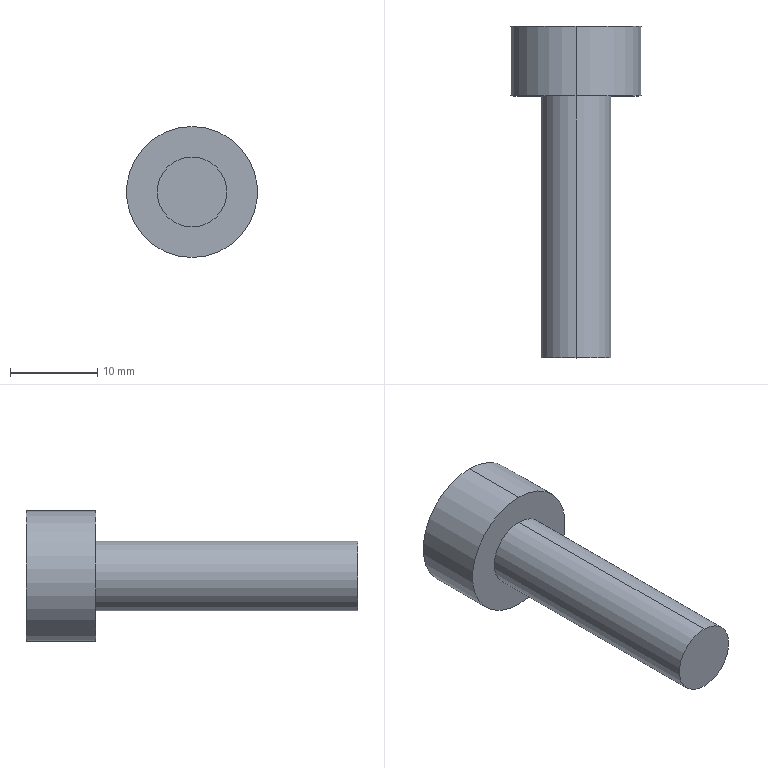Part | STEP file | 1 solid | 14 faces | box 15 x 38 x 15 mm | volume 2735 mm3 | plane 10 | cylinder 4 | commonest cylinder face diameters 8 x2 15 x2
STEP:
#1=CARTESIAN_POINT('',(0.,0.,0.));
#2=DIRECTION('',(0.,0.,1.));
#3=DIRECTION('',(1.,0.,0.));
#4=AXIS2_PLACEMENT_3D('',#1,#2,#3);
#5=CARTESIAN_POINT('',(0.,38.,-7.5));
#6=VERTEX_POINT('',#5);
#7=CARTESIAN_POINT('',(0.,38.,7.5));
#8=VERTEX_POINT('',#7);
#9=CARTESIAN_POINT('',(0.,38.,0.));
#10=DIRECTION('',(0.,-1.,0.));
#11=DIRECTION('',(0.,0.,-1.));
#12=AXIS2_PLACEMENT_3D('',#9,#10,#11);
#13=CIRCLE('',#12,7.5);
#14=CARTESIAN_POINT('',(0.,0.,0.));
#15=DIRECTION('',(0.,-1.,0.));
#16=DIRECTION('',(0.,0.,-1.));
#17=AXIS2_PLACEMENT_3D('',#14,#15,#16);
#18=CYLINDRICAL_SURFACE('',#17,7.5);
#19=CARTESIAN_POINT('',(0.,-38.));
#20=DIRECTION('',(1.,0.));
#21=VECTOR('',#20,1.);
#22=LINE('',#19,#21);
#23=(GEOMETRIC_REPRESENTATION_CONTEXT(2)PARAMETRIC_REPRESENTATION_CONTEXT()REPRESENTATION_CONTEXT('',''));
#24=DEFINITIONAL_REPRESENTATION('',(#22),#23);
#25=PCURVE('',#18,#24);
#26=CARTESIAN_POINT('',(7.5,38.,0.));
#27=DIRECTION('',(0.,1.,0.));
#28=DIRECTION('',(0.,0.,1.));
#29=AXIS2_PLACEMENT_3D('',#26,#27,#28);
#30=PLANE('',#29);
#31=CARTESIAN_POINT('',(-7.5,-7.5));
#32=CARTESIAN_POINT('',(-7.5,5.49));
#33=CARTESIAN_POINT('',(3.75,-1.005));
#34=CARTESIAN_POINT('',(15.,-7.5));
#35=CARTESIAN_POINT('',(3.75,-13.995));
#36=CARTESIAN_POINT('',(-7.5,-20.49));
#37=CARTESIAN_POINT('',(-7.5,-7.5));
#38=(BOUNDED_CURVE()B_SPLINE_CURVE(2,(#31,#32,#33,#34,#35,#36,#37),.UNSPECIFIED.,.T.,.F.)B_SPLINE_CURVE_WITH_KNOTS((1,2,2,2,2,1),(-2.094,0.,2.094,4.189,6.283,8.378),.UNSPECIFIED.)CURVE()GEOMETRIC_REPRESENTATION_ITEM()RATIONAL_B_SPLINE_CURVE((1.,0.5,1.,0.5,1.,0.5,1.))REPRESENTATION_ITEM(''));
#39=(GEOMETRIC_REPRESENTATION_CONTEXT(2)PARAMETRIC_REPRESENTATION_CONTEXT()REPRESENTATION_CONTEXT('',''));
#40=DEFINITIONAL_REPRESENTATION('',(#38),#39);
#41=PCURVE('',#30,#40);
#42=SURFACE_CURVE('',#13,(#25,#41),.PCURVE_S1.);
#43=EDGE_CURVE('',#6,#8,#42,.T.);
#44=ORIENTED_EDGE('',*,*,#43,.T.);
#45=CARTESIAN_POINT('',(0.,30.,7.5));
#46=VERTEX_POINT('',#45);
#47=CARTESIAN_POINT('',(0.,0.,7.5));
#48=DIRECTION('',(0.,-1.,0.));
#49=VECTOR('',#48,1.);
#50=LINE('',#47,#49);
#51=CARTESIAN_POINT('',(3.142,0.));
#52=DIRECTION('',(0.,1.));
#53=VECTOR('',#52,1.);
#54=LINE('',#51,#53);
#55=(GEOMETRIC_REPRESENTATION_CONTEXT(2)PARAMETRIC_REPRESENTATION_CONTEXT()REPRESENTATION_CONTEXT('',''));
#56=DEFINITIONAL_REPRESENTATION('',(#54),#55);
#57=PCURVE('',#18,#56);
#58=CARTESIAN_POINT('',(0.,0.,0.));
#59=DIRECTION('',(0.,-1.,0.));
#60=DIRECTION('',(0.,0.,-1.));
#61=AXIS2_PLACEMENT_3D('',#58,#59,#60);
#62=CYLINDRICAL_SURFACE('',#61,7.5);
#63=CARTESIAN_POINT('',(3.142,0.));
#64=DIRECTION('',(0.,1.));
#65=VECTOR('',#64,1.);
#66=LINE('',#63,#65);
#67=(GEOMETRIC_REPRESENTATION_CONTEXT(2)PARAMETRIC_REPRESENTATION_CONTEXT()REPRESENTATION_CONTEXT('',''));
#68=DEFINITIONAL_REPRESENTATION('',(#66),#67);
#69=PCURVE('',#62,#68);
#70=SURFACE_CURVE('',#50,(#57,#69),.PCURVE_S1.);
#71=EDGE_CURVE('',#8,#46,#70,.T.);
#72=ORIENTED_EDGE('',*,*,#71,.T.);
#73=CARTESIAN_POINT('',(0.,30.,-7.5));
#74=VERTEX_POINT('',#73);
#75=CARTESIAN_POINT('',(0.,30.,0.));
#76=DIRECTION('',(0.,-1.,0.));
#77=DIRECTION('',(0.,0.,-1.));
#78=AXIS2_PLACEMENT_3D('',#75,#76,#77);
#79=CIRCLE('',#78,7.5);
#80=CARTESIAN_POINT('',(0.,-30.));
#81=DIRECTION('',(1.,0.));
#82=VECTOR('',#81,1.);
#83=LINE('',#80,#82);
#84=(GEOMETRIC_REPRESENTATION_CONTEXT(2)PARAMETRIC_REPRESENTATION_CONTEXT()REPRESENTATION_CONTEXT('',''));
#85=DEFINITIONAL_REPRESENTATION('',(#83),#84);
#86=PCURVE('',#18,#85);
#87=CARTESIAN_POINT('',(4.,30.,0.));
#88=DIRECTION('',(0.,-1.,0.));
#89=DIRECTION('',(0.,0.,-1.));
#90=AXIS2_PLACEMENT_3D('',#87,#88,#89);
#91=PLANE('',#90);
#92=CARTESIAN_POINT('',(0.,-4.));
#93=DIRECTION('',(1.,0.));
#94=AXIS2_PLACEMENT_2D('',#92,#93);
#95=CIRCLE('',#94,7.5);
#96=(GEOMETRIC_REPRESENTATION_CONTEXT(2)PARAMETRIC_REPRESENTATION_CONTEXT()REPRESENTATION_CONTEXT('',''));
#97=DEFINITIONAL_REPRESENTATION('',(#95),#96);
#98=PCURVE('',#91,#97);
#99=SURFACE_CURVE('',#79,(#86,#98),.PCURVE_S1.);
#100=EDGE_CURVE('',#74,#46,#99,.T.);
#101=ORIENTED_EDGE('',*,*,#100,.F.);
#102=CARTESIAN_POINT('',(0.,0.,-7.5));
#103=DIRECTION('',(0.,-1.,0.));
#104=VECTOR('',#103,1.);
#105=LINE('',#102,#104);
#106=CARTESIAN_POINT('',(0.,0.));
#107=DIRECTION('',(0.,1.));
#108=VECTOR('',#107,1.);
#109=LINE('',#106,#108);
#110=(GEOMETRIC_REPRESENTATION_CONTEXT(2)PARAMETRIC_REPRESENTATION_CONTEXT()REPRESENTATION_CONTEXT('',''));
#111=DEFINITIONAL_REPRESENTATION('',(#109),#110);
#112=PCURVE('',#18,#111);
#113=CARTESIAN_POINT('',(6.283,0.));
#114=DIRECTION('',(0.,1.));
#115=VECTOR('',#114,1.);
#116=LINE('',#113,#115);
#117=(GEOMETRIC_REPRESENTATION_CONTEXT(2)PARAMETRIC_REPRESENTATION_CONTEXT()REPRESENTATION_CONTEXT('',''));
#118=DEFINITIONAL_REPRESENTATION('',(#116),#117);
#119=PCURVE('',#62,#118);
#120=SURFACE_CURVE('',#105,(#112,#119),.PCURVE_S1.);
#121=EDGE_CURVE('',#6,#74,#120,.T.);
#122=ORIENTED_EDGE('',*,*,#121,.F.);
#123=EDGE_LOOP('',(#44,#72,#101,#122));
#124=FACE_BOUND('',#123,.T.);
#125=ADVANCED_FACE('',(#124),#18,.T.);
#126=CARTESIAN_POINT('',(0.,30.,-4.));
#127=VERTEX_POINT('',#126);
#128=CARTESIAN_POINT('',(0.,30.,4.));
#129=VERTEX_POINT('',#128);
#130=CARTESIAN_POINT('',(0.,30.,0.));
#131=DIRECTION('',(0.,-1.,0.));
#132=DIRECTION('',(0.,0.,-1.));
#133=AXIS2_PLACEMENT_3D('',#130,#131,#132);
#134=CIRCLE('',#133,4.);
#135=CARTESIAN_POINT('',(0.,0.,0.));
#136=DIRECTION('',(0.,-1.,0.));
#137=DIRECTION('',(0.,0.,-1.));
#138=AXIS2_PLACEMENT_3D('',#135,#136,#137);
#139=CYLINDRICAL_SURFACE('',#138,4.);
#140=CARTESIAN_POINT('',(0.,-30.));
#141=DIRECTION('',(1.,0.));
#142=VECTOR('',#141,1.);
#143=LINE('',#140,#142);
#144=(GEOMETRIC_REPRESENTATION_CONTEXT(2)PARAMETRIC_REPRESENTATION_CONTEXT()REPRESENTATION_CONTEXT('',''));
#145=DEFINITIONAL_REPRESENTATION('',(#143),#144);
#146=PCURVE('',#139,#145);
#147=CARTESIAN_POINT('',(0.,-4.));
#148=DIRECTION('',(1.,0.));
#149=AXIS2_PLACEMENT_2D('',#147,#148);
#150=CIRCLE('',#149,4.);
#151=(GEOMETRIC_REPRESENTATION_CONTEXT(2)PARAMETRIC_REPRESENTATION_CONTEXT()REPRESENTATION_CONTEXT('',''));
#152=DEFINITIONAL_REPRESENTATION('',(#150),#151);
#153=PCURVE('',#91,#152);
#154=SURFACE_CURVE('',#134,(#146,#153),.PCURVE_S1.);
#155=EDGE_CURVE('',#127,#129,#154,.T.);
#156=ORIENTED_EDGE('',*,*,#155,.T.);
#157=CARTESIAN_POINT('',(0.,0.,4.));
#158=VERTEX_POINT('',#157);
#159=CARTESIAN_POINT('',(0.,0.,4.));
#160=DIRECTION('',(0.,-1.,0.));
#161=VECTOR('',#160,1.);
#162=LINE('',#159,#161);
#163=CARTESIAN_POINT('',(3.142,0.));
#164=DIRECTION('',(0.,1.));
#165=VECTOR('',#164,1.);
#166=LINE('',#163,#165);
#167=(GEOMETRIC_REPRESENTATION_CONTEXT(2)PARAMETRIC_REPRESENTATION_CONTEXT()REPRESENTATION_CONTEXT('',''));
#168=DEFINITIONAL_REPRESENTATION('',(#166),#167);
#169=PCURVE('',#139,#168);
#170=CARTESIAN_POINT('',(0.,0.,0.));
#171=DIRECTION('',(0.,-1.,0.));
#172=DIRECTION('',(0.,0.,-1.));
#173=AXIS2_PLACEMENT_3D('',#170,#171,#172);
#174=CYLINDRICAL_SURFACE('',#173,4.);
#175=CARTESIAN_POINT('',(3.142,0.));
#176=DIRECTION('',(0.,1.));
#177=VECTOR('',#176,1.);
#178=LINE('',#175,#177);
#179=(GEOMETRIC_REPRESENTATION_CONTEXT(2)PARAMETRIC_REPRESENTATION_CONTEXT()REPRESENTATION_CONTEXT('',''));
#180=DEFINITIONAL_REPRESENTATION('',(#178),#179);
#181=PCURVE('',#174,#180);
#182=SURFACE_CURVE('',#162,(#169,#181),.PCURVE_S1.);
#183=EDGE_CURVE('',#129,#158,#182,.T.);
#184=ORIENTED_EDGE('',*,*,#183,.T.);
#185=CARTESIAN_POINT('',(0.,0.,-4.));
#186=VERTEX_POINT('',#185);
#187=CARTESIAN_POINT('',(0.,0.,0.));
#188=DIRECTION('',(0.,-1.,0.));
#189=DIRECTION('',(0.,0.,-1.));
#190=AXIS2_PLACEMENT_3D('',#187,#188,#189);
#191=CIRCLE('',#190,4.);
#192=CARTESIAN_POINT('',(0.,0.));
#193=DIRECTION('',(1.,0.));
#194=VECTOR('',#193,1.);
#195=LINE('',#192,#194);
#196=(GEOMETRIC_REPRESENTATION_CONTEXT(2)PARAMETRIC_REPRESENTATION_CONTEXT()REPRESENTATION_CONTEXT('',''));
#197=DEFINITIONAL_REPRESENTATION('',(#195),#196);
#198=PCURVE('',#139,#197);
#199=CARTESIAN_POINT('',(0.,0.,0.));
#200=DIRECTION('',(0.,-1.,0.));
#201=DIRECTION('',(0.,0.,-1.));
#202=AXIS2_PLACEMENT_3D('',#199,#200,#201);
#203=PLANE('',#202);
#204=CARTESIAN_POINT('',(0.,0.));
#205=DIRECTION('',(1.,0.));
#206=AXIS2_PLACEMENT_2D('',#204,#205);
#207=CIRCLE('',#206,4.);
#208=(GEOMETRIC_REPRESENTATION_CONTEXT(2)PARAMETRIC_REPRESENTATION_CONTEXT()REPRESENTATION_CONTEXT('',''));
#209=DEFINITIONAL_REPRESENTATION('',(#207),#208);
#210=PCURVE('',#203,#209);
#211=SURFACE_CURVE('',#191,(#198,#210),.PCURVE_S1.);
#212=EDGE_CURVE('',#186,#158,#211,.T.);
#213=ORIENTED_EDGE('',*,*,#212,.F.);
#214=CARTESIAN_POINT('',(0.,0.,-4.));
#215=DIRECTION('',(0.,-1.,0.));
#216=VECTOR('',#215,1.);
#217=LINE('',#214,#216);
#218=CARTESIAN_POINT('',(0.,0.));
#219=DIRECTION('',(0.,1.));
#220=VECTOR('',#219,1.);
#221=LINE('',#218,#220);
#222=(GEOMETRIC_REPRESENTATION_CONTEXT(2)PARAMETRIC_REPRESENTATION_CONTEXT()REPRESENTATION_CONTEXT('',''));
#223=DEFINITIONAL_REPRESENTATION('',(#221),#222);
#224=PCURVE('',#139,#223);
#225=CARTESIAN_POINT('',(6.283,0.));
#226=DIRECTION('',(0.,1.));
#227=VECTOR('',#226,1.);
#228=LINE('',#225,#227);
#229=(GEOMETRIC_REPRESENTATION_CONTEXT(2)PARAMETRIC_REPRESENTATION_CONTEXT()REPRESENTATION_CONTEXT('',''));
#230=DEFINITIONAL_REPRESENTATION('',(#228),#229);
#231=PCURVE('',#174,#230);
#232=SURFACE_CURVE('',#217,(#224,#231),.PCURVE_S1.);
#233=EDGE_CURVE('',#127,#186,#232,.T.);
#234=ORIENTED_EDGE('',*,*,#233,.F.);
#235=EDGE_LOOP('',(#156,#184,#213,#234));
#236=FACE_BOUND('',#235,.T.);
#237=ADVANCED_FACE('',(#236),#139,.T.);
#238=ORIENTED_EDGE('',*,*,#212,.T.);
#239=CARTESIAN_POINT('',(0.,0.,0.));
#240=DIRECTION('',(0.,-1.,0.));
#241=DIRECTION('',(0.,0.,-1.));
#242=AXIS2_PLACEMENT_3D('',#239,#240,#241);
#243=CIRCLE('',#242,4.);
#244=CARTESIAN_POINT('',(0.,0.));
#245=DIRECTION('',(1.,0.));
#246=AXIS2_PLACEMENT_2D('',#244,#245);
#247=CIRCLE('',#246,4.);
#248=(GEOMETRIC_REPRESENTATION_CONTEXT(2)PARAMETRIC_REPRESENTATION_CONTEXT()REPRESENTATION_CONTEXT('',''));
#249=DEFINITIONAL_REPRESENTATION('',(#247),#248);
#250=PCURVE('',#203,#249);
#251=CARTESIAN_POINT('',(0.,0.));
#252=DIRECTION('',(1.,0.));
#253=VECTOR('',#252,1.);
#254=LINE('',#251,#253);
#255=(GEOMETRIC_REPRESENTATION_CONTEXT(2)PARAMETRIC_REPRESENTATION_CONTEXT()REPRESENTATION_CONTEXT('',''));
#256=DEFINITIONAL_REPRESENTATION('',(#254),#255);
#257=PCURVE('',#174,#256);
#258=SURFACE_CURVE('',#243,(#250,#257),.PCURVE_S1.);
#259=EDGE_CURVE('',#158,#186,#258,.T.);
#260=ORIENTED_EDGE('',*,*,#259,.T.);
#261=EDGE_LOOP('',(#238,#260));
#262=FACE_BOUND('',#261,.T.);
#263=ADVANCED_FACE('',(#262),#203,.T.);
#264=ORIENTED_EDGE('',*,*,#183,.F.);
#265=CARTESIAN_POINT('',(0.,30.,0.));
#266=DIRECTION('',(0.,-1.,0.));
#267=DIRECTION('',(0.,0.,-1.));
#268=AXIS2_PLACEMENT_3D('',#265,#266,#267);
#269=CIRCLE('',#268,4.);
#270=CARTESIAN_POINT('',(0.,-30.));
#271=DIRECTION('',(1.,0.));
#272=VECTOR('',#271,1.);
#273=LINE('',#270,#272);
#274=(GEOMETRIC_REPRESENTATION_CONTEXT(2)PARAMETRIC_REPRESENTATION_CONTEXT()REPRESENTATION_CONTEXT('',''));
#275=DEFINITIONAL_REPRESENTATION('',(#273),#274);
#276=PCURVE('',#174,#275);
#277=CARTESIAN_POINT('',(0.,-4.));
#278=DIRECTION('',(1.,0.));
#279=AXIS2_PLACEMENT_2D('',#277,#278);
#280=CIRCLE('',#279,4.);
#281=(GEOMETRIC_REPRESENTATION_CONTEXT(2)PARAMETRIC_REPRESENTATION_CONTEXT()REPRESENTATION_CONTEXT('',''));
#282=DEFINITIONAL_REPRESENTATION('',(#280),#281);
#283=PCURVE('',#91,#282);
#284=SURFACE_CURVE('',#269,(#276,#283),.PCURVE_S1.);
#285=EDGE_CURVE('',#129,#127,#284,.T.);
#286=ORIENTED_EDGE('',*,*,#285,.T.);
#287=ORIENTED_EDGE('',*,*,#233,.T.);
#288=ORIENTED_EDGE('',*,*,#259,.F.);
#289=EDGE_LOOP('',(#264,#286,#287,#288));
#290=FACE_BOUND('',#289,.T.);
#291=ADVANCED_FACE('',(#290),#174,.T.);
#292=ORIENTED_EDGE('',*,*,#100,.T.);
#293=CARTESIAN_POINT('',(0.,30.,0.));
#294=DIRECTION('',(0.,-1.,0.));
#295=DIRECTION('',(0.,0.,-1.));
#296=AXIS2_PLACEMENT_3D('',#293,#294,#295);
#297=CIRCLE('',#296,7.5);
#298=CARTESIAN_POINT('',(0.,-4.));
#299=DIRECTION('',(1.,0.));
#300=AXIS2_PLACEMENT_2D('',#298,#299);
#301=CIRCLE('',#300,7.5);
#302=(GEOMETRIC_REPRESENTATION_CONTEXT(2)PARAMETRIC_REPRESENTATION_CONTEXT()REPRESENTATION_CONTEXT('',''));
#303=DEFINITIONAL_REPRESENTATION('',(#301),#302);
#304=PCURVE('',#91,#303);
#305=CARTESIAN_POINT('',(0.,-30.));
#306=DIRECTION('',(1.,0.));
#307=VECTOR('',#306,1.);
#308=LINE('',#305,#307);
#309=(GEOMETRIC_REPRESENTATION_CONTEXT(2)PARAMETRIC_REPRESENTATION_CONTEXT()REPRESENTATION_CONTEXT('',''));
#310=DEFINITIONAL_REPRESENTATION('',(#308),#309);
#311=PCURVE('',#62,#310);
#312=SURFACE_CURVE('',#297,(#304,#311),.PCURVE_S1.);
#313=EDGE_CURVE('',#46,#74,#312,.T.);
#314=ORIENTED_EDGE('',*,*,#313,.T.);
#315=EDGE_LOOP('',(#292,#314));
#316=FACE_BOUND('',#315,.T.);
#317=ORIENTED_EDGE('',*,*,#155,.F.);
#318=ORIENTED_EDGE('',*,*,#285,.F.);
#319=EDGE_LOOP('',(#317,#318));
#320=FACE_BOUND('',#319,.T.);
#321=ADVANCED_FACE('',(#316,#320),#91,.T.);
#322=ORIENTED_EDGE('',*,*,#71,.F.);
#323=CARTESIAN_POINT('',(0.,38.,0.));
#324=DIRECTION('',(0.,-1.,0.));
#325=DIRECTION('',(0.,0.,-1.));
#326=AXIS2_PLACEMENT_3D('',#323,#324,#325);
#327=CIRCLE('',#326,7.5);
#328=CARTESIAN_POINT('',(0.,-38.));
#329=DIRECTION('',(1.,0.));
#330=VECTOR('',#329,1.);
#331=LINE('',#328,#330);
#332=(GEOMETRIC_REPRESENTATION_CONTEXT(2)PARAMETRIC_REPRESENTATION_CONTEXT()REPRESENTATION_CONTEXT('',''));
#333=DEFINITIONAL_REPRESENTATION('',(#331),#332);
#334=PCURVE('',#62,#333);
#335=CARTESIAN_POINT('',(-7.5,-7.5));
#336=CARTESIAN_POINT('',(-7.5,5.49));
#337=CARTESIAN_POINT('',(3.75,-1.005));
#338=CARTESIAN_POINT('',(15.,-7.5));
#339=CARTESIAN_POINT('',(3.75,-13.995));
#340=CARTESIAN_POINT('',(-7.5,-20.49));
#341=CARTESIAN_POINT('',(-7.5,-7.5));
#342=(BOUNDED_CURVE()B_SPLINE_CURVE(2,(#335,#336,#337,#338,#339,#340,#341),.UNSPECIFIED.,.T.,.F.)B_SPLINE_CURVE_WITH_KNOTS((1,2,2,2,2,1),(-2.094,0.,2.094,4.189,6.283,8.378),.UNSPECIFIED.)CURVE()GEOMETRIC_REPRESENTATION_ITEM()RATIONAL_B_SPLINE_CURVE((1.,0.5,1.,0.5,1.,0.5,1.))REPRESENTATION_ITEM(''));
#343=(GEOMETRIC_REPRESENTATION_CONTEXT(2)PARAMETRIC_REPRESENTATION_CONTEXT()REPRESENTATION_CONTEXT('',''));
#344=DEFINITIONAL_REPRESENTATION('',(#342),#343);
#345=PCURVE('',#30,#344);
#346=SURFACE_CURVE('',#327,(#334,#345),.PCURVE_S1.);
#347=EDGE_CURVE('',#8,#6,#346,.T.);
#348=ORIENTED_EDGE('',*,*,#347,.T.);
#349=ORIENTED_EDGE('',*,*,#121,.T.);
#350=ORIENTED_EDGE('',*,*,#313,.F.);
#351=EDGE_LOOP('',(#322,#348,#349,#350));
#352=FACE_BOUND('',#351,.T.);
#353=ADVANCED_FACE('',(#352),#62,.T.);
#354=CARTESIAN_POINT('',(1.732,38.,3.));
#355=VERTEX_POINT('',#354);
#356=CARTESIAN_POINT('',(3.464,38.,0.));
#357=VERTEX_POINT('',#356);
#358=CARTESIAN_POINT('',(1.732,38.,3.));
#359=DIRECTION('',(0.5,0.,-0.866));
#360=VECTOR('',#359,1.);
#361=LINE('',#358,#360);
#362=CARTESIAN_POINT('',(3.,-5.768));
#363=DIRECTION('',(-0.866,0.5));
#364=VECTOR('',#363,1.);
#365=LINE('',#362,#364);
#366=(GEOMETRIC_REPRESENTATION_CONTEXT(2)PARAMETRIC_REPRESENTATION_CONTEXT()REPRESENTATION_CONTEXT('',''));
#367=DEFINITIONAL_REPRESENTATION('',(#365),#366);
#368=PCURVE('',#30,#367);
#369=CARTESIAN_POINT('',(1.732,32.,3.));
#370=DIRECTION('',(0.866,0.,0.5));
#371=DIRECTION('',(0.5,0.,-0.866));
#372=AXIS2_PLACEMENT_3D('',#369,#370,#371);
#373=PLANE('',#372);
#374=CARTESIAN_POINT('',(0.,6.));
#375=DIRECTION('',(1.,0.));
#376=VECTOR('',#375,1.);
#377=LINE('',#374,#376);
#378=(GEOMETRIC_REPRESENTATION_CONTEXT(2)PARAMETRIC_REPRESENTATION_CONTEXT()REPRESENTATION_CONTEXT('',''));
#379=DEFINITIONAL_REPRESENTATION('',(#377),#378);
#380=PCURVE('',#373,#379);
#381=SURFACE_CURVE('',#361,(#368,#380),.PCURVE_S1.);
#382=EDGE_CURVE('',#355,#357,#381,.T.);
#383=ORIENTED_EDGE('',*,*,#382,.F.);
#384=CARTESIAN_POINT('',(-1.732,38.,3.));
#385=VERTEX_POINT('',#384);
#386=CARTESIAN_POINT('',(-1.732,38.,3.));
#387=DIRECTION('',(1.,0.,0.));
#388=VECTOR('',#387,1.);
#389=LINE('',#386,#388);
#390=CARTESIAN_POINT('',(3.,-9.232));
#391=DIRECTION('',(0.,1.));
#392=VECTOR('',#391,1.);
#393=LINE('',#390,#392);
#394=(GEOMETRIC_REPRESENTATION_CONTEXT(2)PARAMETRIC_REPRESENTATION_CONTEXT()REPRESENTATION_CONTEXT('',''));
#395=DEFINITIONAL_REPRESENTATION('',(#393),#394);
#396=PCURVE('',#30,#395);
#397=CARTESIAN_POINT('',(-1.732,32.,3.));
#398=DIRECTION('',(0.,0.,1.));
#399=DIRECTION('',(1.,0.,0.));
#400=AXIS2_PLACEMENT_3D('',#397,#398,#399);
#401=PLANE('',#400);
#402=CARTESIAN_POINT('',(0.,6.));
#403=DIRECTION('',(1.,0.));
#404=VECTOR('',#403,1.);
#405=LINE('',#402,#404);
#406=(GEOMETRIC_REPRESENTATION_CONTEXT(2)PARAMETRIC_REPRESENTATION_CONTEXT()REPRESENTATION_CONTEXT('',''));
#407=DEFINITIONAL_REPRESENTATION('',(#405),#406);
#408=PCURVE('',#401,#407);
#409=SURFACE_CURVE('',#389,(#396,#408),.PCURVE_S1.);
#410=EDGE_CURVE('',#385,#355,#409,.T.);
#411=ORIENTED_EDGE('',*,*,#410,.F.);
#412=CARTESIAN_POINT('',(-3.464,38.,0.));
#413=VERTEX_POINT('',#412);
#414=CARTESIAN_POINT('',(-3.464,38.,0.));
#415=DIRECTION('',(0.5,0.,0.866));
#416=VECTOR('',#415,1.);
#417=LINE('',#414,#416);
#418=CARTESIAN_POINT('',(0.,-10.964));
#419=DIRECTION('',(0.866,0.5));
#420=VECTOR('',#419,1.);
#421=LINE('',#418,#420);
#422=(GEOMETRIC_REPRESENTATION_CONTEXT(2)PARAMETRIC_REPRESENTATION_CONTEXT()REPRESENTATION_CONTEXT('',''));
#423=DEFINITIONAL_REPRESENTATION('',(#421),#422);
#424=PCURVE('',#30,#423);
#425=CARTESIAN_POINT('',(-3.464,32.,0.));
#426=DIRECTION('',(-0.866,0.,0.5));
#427=DIRECTION('',(0.5,0.,0.866));
#428=AXIS2_PLACEMENT_3D('',#425,#426,#427);
#429=PLANE('',#428);
#430=CARTESIAN_POINT('',(0.,6.));
#431=DIRECTION('',(1.,0.));
#432=VECTOR('',#431,1.);
#433=LINE('',#430,#432);
#434=(GEOMETRIC_REPRESENTATION_CONTEXT(2)PARAMETRIC_REPRESENTATION_CONTEXT()REPRESENTATION_CONTEXT('',''));
#435=DEFINITIONAL_REPRESENTATION('',(#433),#434);
#436=PCURVE('',#429,#435);
#437=SURFACE_CURVE('',#417,(#424,#436),.PCURVE_S1.);
#438=EDGE_CURVE('',#413,#385,#437,.T.);
#439=ORIENTED_EDGE('',*,*,#438,.F.);
#440=CARTESIAN_POINT('',(-1.732,38.,-3.));
#441=VERTEX_POINT('',#440);
#442=CARTESIAN_POINT('',(-1.732,38.,-3.));
#443=DIRECTION('',(-0.5,0.,0.866));
#444=VECTOR('',#443,1.);
#445=LINE('',#442,#444);
#446=CARTESIAN_POINT('',(-3.,-9.232));
#447=DIRECTION('',(0.866,-0.5));
#448=VECTOR('',#447,1.);
#449=LINE('',#446,#448);
#450=(GEOMETRIC_REPRESENTATION_CONTEXT(2)PARAMETRIC_REPRESENTATION_CONTEXT()REPRESENTATION_CONTEXT('',''));
#451=DEFINITIONAL_REPRESENTATION('',(#449),#450);
#452=PCURVE('',#30,#451);
#453=CARTESIAN_POINT('',(-1.732,32.,-3.));
#454=DIRECTION('',(-0.866,0.,-0.5));
#455=DIRECTION('',(-0.5,0.,0.866));
#456=AXIS2_PLACEMENT_3D('',#453,#454,#455);
#457=PLANE('',#456);
#458=CARTESIAN_POINT('',(0.,6.));
#459=DIRECTION('',(1.,0.));
#460=VECTOR('',#459,1.);
#461=LINE('',#458,#460);
#462=(GEOMETRIC_REPRESENTATION_CONTEXT(2)PARAMETRIC_REPRESENTATION_CONTEXT()REPRESENTATION_CONTEXT('',''));
#463=DEFINITIONAL_REPRESENTATION('',(#461),#462);
#464=PCURVE('',#457,#463);
#465=SURFACE_CURVE('',#445,(#452,#464),.PCURVE_S1.);
#466=EDGE_CURVE('',#441,#413,#465,.T.);
#467=ORIENTED_EDGE('',*,*,#466,.F.);
#468=CARTESIAN_POINT('',(1.732,38.,-3.));
#469=VERTEX_POINT('',#468);
#470=CARTESIAN_POINT('',(1.732,38.,-3.));
#471=DIRECTION('',(-1.,0.,0.));
#472=VECTOR('',#471,1.);
#473=LINE('',#470,#472);
#474=CARTESIAN_POINT('',(-3.,-5.768));
#475=DIRECTION('',(0.,-1.));
#476=VECTOR('',#475,1.);
#477=LINE('',#474,#476);
#478=(GEOMETRIC_REPRESENTATION_CONTEXT(2)PARAMETRIC_REPRESENTATION_CONTEXT()REPRESENTATION_CONTEXT('',''));
#479=DEFINITIONAL_REPRESENTATION('',(#477),#478);
#480=PCURVE('',#30,#479);
#481=CARTESIAN_POINT('',(1.732,32.,-3.));
#482=DIRECTION('',(0.,0.,-1.));
#483=DIRECTION('',(-1.,0.,0.));
#484=AXIS2_PLACEMENT_3D('',#481,#482,#483);
#485=PLANE('',#484);
#486=CARTESIAN_POINT('',(0.,6.));
#487=DIRECTION('',(1.,0.));
#488=VECTOR('',#487,1.);
#489=LINE('',#486,#488);
#490=(GEOMETRIC_REPRESENTATION_CONTEXT(2)PARAMETRIC_REPRESENTATION_CONTEXT()REPRESENTATION_CONTEXT('',''));
#491=DEFINITIONAL_REPRESENTATION('',(#489),#490);
#492=PCURVE('',#485,#491);
#493=SURFACE_CURVE('',#473,(#480,#492),.PCURVE_S1.);
#494=EDGE_CURVE('',#469,#441,#493,.T.);
#495=ORIENTED_EDGE('',*,*,#494,.F.);
#496=CARTESIAN_POINT('',(3.464,38.,0.));
#497=DIRECTION('',(-0.5,0.,-0.866));
#498=VECTOR('',#497,1.);
#499=LINE('',#496,#498);
#500=CARTESIAN_POINT('',(0.,-4.036));
#501=DIRECTION('',(-0.866,-0.5));
#502=VECTOR('',#501,1.);
#503=LINE('',#500,#502);
#504=(GEOMETRIC_REPRESENTATION_CONTEXT(2)PARAMETRIC_REPRESENTATION_CONTEXT()REPRESENTATION_CONTEXT('',''));
#505=DEFINITIONAL_REPRESENTATION('',(#503),#504);
#506=PCURVE('',#30,#505);
#507=CARTESIAN_POINT('',(3.464,32.,0.));
#508=DIRECTION('',(0.866,0.,-0.5));
#509=DIRECTION('',(-0.5,0.,-0.866));
#510=AXIS2_PLACEMENT_3D('',#507,#508,#509);
#511=PLANE('',#510);
#512=CARTESIAN_POINT('',(0.,6.));
#513=DIRECTION('',(1.,0.));
#514=VECTOR('',#513,1.);
#515=LINE('',#512,#514);
#516=(GEOMETRIC_REPRESENTATION_CONTEXT(2)PARAMETRIC_REPRESENTATION_CONTEXT()REPRESENTATION_CONTEXT('',''));
#517=DEFINITIONAL_REPRESENTATION('',(#515),#516);
#518=PCURVE('',#511,#517);
#519=SURFACE_CURVE('',#499,(#506,#518),.PCURVE_S1.);
#520=EDGE_CURVE('',#357,#469,#519,.T.);
#521=ORIENTED_EDGE('',*,*,#520,.F.);
#522=EDGE_LOOP('',(#383,#411,#439,#467,#495,#521));
#523=FACE_BOUND('',#522,.T.);
#524=ORIENTED_EDGE('',*,*,#43,.F.);
#525=ORIENTED_EDGE('',*,*,#347,.F.);
#526=EDGE_LOOP('',(#524,#525));
#527=FACE_BOUND('',#526,.T.);
#528=ADVANCED_FACE('',(#523,#527),#30,.T.);
#529=ORIENTED_EDGE('',*,*,#382,.T.);
#530=CARTESIAN_POINT('',(3.464,32.,0.));
#531=VERTEX_POINT('',#530);
#532=CARTESIAN_POINT('',(3.464,32.,0.));
#533=DIRECTION('',(0.,1.,0.));
#534=VECTOR('',#533,1.);
#535=LINE('',#532,#534);
#536=CARTESIAN_POINT('',(3.464,0.));
#537=DIRECTION('',(0.,1.));
#538=VECTOR('',#537,1.);
#539=LINE('',#536,#538);
#540=(GEOMETRIC_REPRESENTATION_CONTEXT(2)PARAMETRIC_REPRESENTATION_CONTEXT()REPRESENTATION_CONTEXT('',''));
#541=DEFINITIONAL_REPRESENTATION('',(#539),#540);
#542=PCURVE('',#373,#541);
#543=CARTESIAN_POINT('',(0.,0.));
#544=DIRECTION('',(0.,1.));
#545=VECTOR('',#544,1.);
#546=LINE('',#543,#545);
#547=(GEOMETRIC_REPRESENTATION_CONTEXT(2)PARAMETRIC_REPRESENTATION_CONTEXT()REPRESENTATION_CONTEXT('',''));
#548=DEFINITIONAL_REPRESENTATION('',(#546),#547);
#549=PCURVE('',#511,#548);
#550=SURFACE_CURVE('',#535,(#542,#549),.PCURVE_S1.);
#551=EDGE_CURVE('',#531,#357,#550,.T.);
#552=ORIENTED_EDGE('',*,*,#551,.F.);
#553=CARTESIAN_POINT('',(1.732,32.,3.));
#554=VERTEX_POINT('',#553);
#555=CARTESIAN_POINT('',(1.732,32.,3.));
#556=DIRECTION('',(0.5,0.,-0.866));
#557=VECTOR('',#556,1.);
#558=LINE('',#555,#557);
#559=CARTESIAN_POINT('',(0.,0.));
#560=DIRECTION('',(1.,0.));
#561=VECTOR('',#560,1.);
#562=LINE('',#559,#561);
#563=(GEOMETRIC_REPRESENTATION_CONTEXT(2)PARAMETRIC_REPRESENTATION_CONTEXT()REPRESENTATION_CONTEXT('',''));
#564=DEFINITIONAL_REPRESENTATION('',(#562),#563);
#565=PCURVE('',#373,#564);
#566=CARTESIAN_POINT('',(0.,32.,0.));
#567=DIRECTION('',(0.,1.,0.));
#568=DIRECTION('',(0.,0.,1.));
#569=AXIS2_PLACEMENT_3D('',#566,#567,#568);
#570=PLANE('',#569);
#571=CARTESIAN_POINT('',(3.,1.732));
#572=DIRECTION('',(-0.866,0.5));
#573=VECTOR('',#572,1.);
#574=LINE('',#571,#573);
#575=(GEOMETRIC_REPRESENTATION_CONTEXT(2)PARAMETRIC_REPRESENTATION_CONTEXT()REPRESENTATION_CONTEXT('',''));
#576=DEFINITIONAL_REPRESENTATION('',(#574),#575);
#577=PCURVE('',#570,#576);
#578=SURFACE_CURVE('',#558,(#565,#577),.PCURVE_S1.);
#579=EDGE_CURVE('',#554,#531,#578,.T.);
#580=ORIENTED_EDGE('',*,*,#579,.F.);
#581=CARTESIAN_POINT('',(1.732,32.,3.));
#582=DIRECTION('',(0.,1.,0.));
#583=VECTOR('',#582,1.);
#584=LINE('',#581,#583);
#585=CARTESIAN_POINT('',(0.,0.));
#586=DIRECTION('',(0.,1.));
#587=VECTOR('',#586,1.);
#588=LINE('',#585,#587);
#589=(GEOMETRIC_REPRESENTATION_CONTEXT(2)PARAMETRIC_REPRESENTATION_CONTEXT()REPRESENTATION_CONTEXT('',''));
#590=DEFINITIONAL_REPRESENTATION('',(#588),#589);
#591=PCURVE('',#373,#590);
#592=CARTESIAN_POINT('',(3.464,0.));
#593=DIRECTION('',(0.,1.));
#594=VECTOR('',#593,1.);
#595=LINE('',#592,#594);
#596=(GEOMETRIC_REPRESENTATION_CONTEXT(2)PARAMETRIC_REPRESENTATION_CONTEXT()REPRESENTATION_CONTEXT('',''));
#597=DEFINITIONAL_REPRESENTATION('',(#595),#596);
#598=PCURVE('',#401,#597);
#599=SURFACE_CURVE('',#584,(#591,#598),.PCURVE_S1.);
#600=EDGE_CURVE('',#554,#355,#599,.T.);
#601=ORIENTED_EDGE('',*,*,#600,.T.);
#602=EDGE_LOOP('',(#529,#552,#580,#601));
#603=FACE_BOUND('',#602,.T.);
#604=ADVANCED_FACE('',(#603),#373,.F.);
#605=ORIENTED_EDGE('',*,*,#410,.T.);
#606=ORIENTED_EDGE('',*,*,#600,.F.);
#607=CARTESIAN_POINT('',(-1.732,32.,3.));
#608=VERTEX_POINT('',#607);
#609=CARTESIAN_POINT('',(-1.732,32.,3.));
#610=DIRECTION('',(1.,0.,0.));
#611=VECTOR('',#610,1.);
#612=LINE('',#609,#611);
#613=CARTESIAN_POINT('',(0.,0.));
#614=DIRECTION('',(1.,0.));
#615=VECTOR('',#614,1.);
#616=LINE('',#613,#615);
#617=(GEOMETRIC_REPRESENTATION_CONTEXT(2)PARAMETRIC_REPRESENTATION_CONTEXT()REPRESENTATION_CONTEXT('',''));
#618=DEFINITIONAL_REPRESENTATION('',(#616),#617);
#619=PCURVE('',#401,#618);
#620=CARTESIAN_POINT('',(3.,-1.732));
#621=DIRECTION('',(0.,1.));
#622=VECTOR('',#621,1.);
#623=LINE('',#620,#622);
#624=(GEOMETRIC_REPRESENTATION_CONTEXT(2)PARAMETRIC_REPRESENTATION_CONTEXT()REPRESENTATION_CONTEXT('',''));
#625=DEFINITIONAL_REPRESENTATION('',(#623),#624);
#626=PCURVE('',#570,#625);
#627=SURFACE_CURVE('',#612,(#619,#626),.PCURVE_S1.);
#628=EDGE_CURVE('',#608,#554,#627,.T.);
#629=ORIENTED_EDGE('',*,*,#628,.F.);
#630=CARTESIAN_POINT('',(-1.732,32.,3.));
#631=DIRECTION('',(0.,1.,0.));
#632=VECTOR('',#631,1.);
#633=LINE('',#630,#632);
#634=CARTESIAN_POINT('',(0.,0.));
#635=DIRECTION('',(0.,1.));
#636=VECTOR('',#635,1.);
#637=LINE('',#634,#636);
#638=(GEOMETRIC_REPRESENTATION_CONTEXT(2)PARAMETRIC_REPRESENTATION_CONTEXT()REPRESENTATION_CONTEXT('',''));
#639=DEFINITIONAL_REPRESENTATION('',(#637),#638);
#640=PCURVE('',#401,#639);
#641=CARTESIAN_POINT('',(3.464,0.));
#642=DIRECTION('',(0.,1.));
#643=VECTOR('',#642,1.);
#644=LINE('',#641,#643);
#645=(GEOMETRIC_REPRESENTATION_CONTEXT(2)PARAMETRIC_REPRESENTATION_CONTEXT()REPRESENTATION_CONTEXT('',''));
#646=DEFINITIONAL_REPRESENTATION('',(#644),#645);
#647=PCURVE('',#429,#646);
#648=SURFACE_CURVE('',#633,(#640,#647),.PCURVE_S1.);
#649=EDGE_CURVE('',#608,#385,#648,.T.);
#650=ORIENTED_EDGE('',*,*,#649,.T.);
#651=EDGE_LOOP('',(#605,#606,#629,#650));
#652=FACE_BOUND('',#651,.T.);
#653=ADVANCED_FACE('',(#652),#401,.F.);
#654=ORIENTED_EDGE('',*,*,#438,.T.);
#655=ORIENTED_EDGE('',*,*,#649,.F.);
#656=CARTESIAN_POINT('',(-3.464,32.,0.));
#657=VERTEX_POINT('',#656);
#658=CARTESIAN_POINT('',(-3.464,32.,0.));
#659=DIRECTION('',(0.5,0.,0.866));
#660=VECTOR('',#659,1.);
#661=LINE('',#658,#660);
#662=CARTESIAN_POINT('',(0.,0.));
#663=DIRECTION('',(1.,0.));
#664=VECTOR('',#663,1.);
#665=LINE('',#662,#664);
#666=(GEOMETRIC_REPRESENTATION_CONTEXT(2)PARAMETRIC_REPRESENTATION_CONTEXT()REPRESENTATION_CONTEXT('',''));
#667=DEFINITIONAL_REPRESENTATION('',(#665),#666);
#668=PCURVE('',#429,#667);
#669=CARTESIAN_POINT('',(0.,-3.464));
#670=DIRECTION('',(0.866,0.5));
#671=VECTOR('',#670,1.);
#672=LINE('',#669,#671);
#673=(GEOMETRIC_REPRESENTATION_CONTEXT(2)PARAMETRIC_REPRESENTATION_CONTEXT()REPRESENTATION_CONTEXT('',''));
#674=DEFINITIONAL_REPRESENTATION('',(#672),#673);
#675=PCURVE('',#570,#674);
#676=SURFACE_CURVE('',#661,(#668,#675),.PCURVE_S1.);
#677=EDGE_CURVE('',#657,#608,#676,.T.);
#678=ORIENTED_EDGE('',*,*,#677,.F.);
#679=CARTESIAN_POINT('',(-3.464,32.,0.));
#680=DIRECTION('',(0.,1.,0.));
#681=VECTOR('',#680,1.);
#682=LINE('',#679,#681);
#683=CARTESIAN_POINT('',(0.,0.));
#684=DIRECTION('',(0.,1.));
#685=VECTOR('',#684,1.);
#686=LINE('',#683,#685);
#687=(GEOMETRIC_REPRESENTATION_CONTEXT(2)PARAMETRIC_REPRESENTATION_CONTEXT()REPRESENTATION_CONTEXT('',''));
#688=DEFINITIONAL_REPRESENTATION('',(#686),#687);
#689=PCURVE('',#429,#688);
#690=CARTESIAN_POINT('',(3.464,0.));
#691=DIRECTION('',(0.,1.));
#692=VECTOR('',#691,1.);
#693=LINE('',#690,#692);
#694=(GEOMETRIC_REPRESENTATION_CONTEXT(2)PARAMETRIC_REPRESENTATION_CONTEXT()REPRESENTATION_CONTEXT('',''));
#695=DEFINITIONAL_REPRESENTATION('',(#693),#694);
#696=PCURVE('',#457,#695);
#697=SURFACE_CURVE('',#682,(#689,#696),.PCURVE_S1.);
#698=EDGE_CURVE('',#657,#413,#697,.T.);
#699=ORIENTED_EDGE('',*,*,#698,.T.);
#700=EDGE_LOOP('',(#654,#655,#678,#699));
#701=FACE_BOUND('',#700,.T.);
#702=ADVANCED_FACE('',(#701),#429,.F.);
#703=ORIENTED_EDGE('',*,*,#466,.T.);
#704=ORIENTED_EDGE('',*,*,#698,.F.);
#705=CARTESIAN_POINT('',(-1.732,32.,-3.));
#706=VERTEX_POINT('',#705);
#707=CARTESIAN_POINT('',(-1.732,32.,-3.));
#708=DIRECTION('',(-0.5,0.,0.866));
#709=VECTOR('',#708,1.);
#710=LINE('',#707,#709);
#711=CARTESIAN_POINT('',(0.,0.));
#712=DIRECTION('',(1.,0.));
#713=VECTOR('',#712,1.);
#714=LINE('',#711,#713);
#715=(GEOMETRIC_REPRESENTATION_CONTEXT(2)PARAMETRIC_REPRESENTATION_CONTEXT()REPRESENTATION_CONTEXT('',''));
#716=DEFINITIONAL_REPRESENTATION('',(#714),#715);
#717=PCURVE('',#457,#716);
#718=CARTESIAN_POINT('',(-3.,-1.732));
#719=DIRECTION('',(0.866,-0.5));
#720=VECTOR('',#719,1.);
#721=LINE('',#718,#720);
#722=(GEOMETRIC_REPRESENTATION_CONTEXT(2)PARAMETRIC_REPRESENTATION_CONTEXT()REPRESENTATION_CONTEXT('',''));
#723=DEFINITIONAL_REPRESENTATION('',(#721),#722);
#724=PCURVE('',#570,#723);
#725=SURFACE_CURVE('',#710,(#717,#724),.PCURVE_S1.);
#726=EDGE_CURVE('',#706,#657,#725,.T.);
#727=ORIENTED_EDGE('',*,*,#726,.F.);
#728=CARTESIAN_POINT('',(-1.732,32.,-3.));
#729=DIRECTION('',(0.,1.,0.));
#730=VECTOR('',#729,1.);
#731=LINE('',#728,#730);
#732=CARTESIAN_POINT('',(0.,0.));
#733=DIRECTION('',(0.,1.));
#734=VECTOR('',#733,1.);
#735=LINE('',#732,#734);
#736=(GEOMETRIC_REPRESENTATION_CONTEXT(2)PARAMETRIC_REPRESENTATION_CONTEXT()REPRESENTATION_CONTEXT('',''));
#737=DEFINITIONAL_REPRESENTATION('',(#735),#736);
#738=PCURVE('',#457,#737);
#739=CARTESIAN_POINT('',(3.464,0.));
#740=DIRECTION('',(0.,1.));
#741=VECTOR('',#740,1.);
#742=LINE('',#739,#741);
#743=(GEOMETRIC_REPRESENTATION_CONTEXT(2)PARAMETRIC_REPRESENTATION_CONTEXT()REPRESENTATION_CONTEXT('',''));
#744=DEFINITIONAL_REPRESENTATION('',(#742),#743);
#745=PCURVE('',#485,#744);
#746=SURFACE_CURVE('',#731,(#738,#745),.PCURVE_S1.);
#747=EDGE_CURVE('',#706,#441,#746,.T.);
#748=ORIENTED_EDGE('',*,*,#747,.T.);
#749=EDGE_LOOP('',(#703,#704,#727,#748));
#750=FACE_BOUND('',#749,.T.);
#751=ADVANCED_FACE('',(#750),#457,.F.);
#752=ORIENTED_EDGE('',*,*,#494,.T.);
#753=ORIENTED_EDGE('',*,*,#747,.F.);
#754=CARTESIAN_POINT('',(1.732,32.,-3.));
#755=VERTEX_POINT('',#754);
#756=CARTESIAN_POINT('',(1.732,32.,-3.));
#757=DIRECTION('',(-1.,0.,0.));
#758=VECTOR('',#757,1.);
#759=LINE('',#756,#758);
#760=CARTESIAN_POINT('',(0.,0.));
#761=DIRECTION('',(1.,0.));
#762=VECTOR('',#761,1.);
#763=LINE('',#760,#762);
#764=(GEOMETRIC_REPRESENTATION_CONTEXT(2)PARAMETRIC_REPRESENTATION_CONTEXT()REPRESENTATION_CONTEXT('',''));
#765=DEFINITIONAL_REPRESENTATION('',(#763),#764);
#766=PCURVE('',#485,#765);
#767=CARTESIAN_POINT('',(-3.,1.732));
#768=DIRECTION('',(0.,-1.));
#769=VECTOR('',#768,1.);
#770=LINE('',#767,#769);
#771=(GEOMETRIC_REPRESENTATION_CONTEXT(2)PARAMETRIC_REPRESENTATION_CONTEXT()REPRESENTATION_CONTEXT('',''));
#772=DEFINITIONAL_REPRESENTATION('',(#770),#771);
#773=PCURVE('',#570,#772);
#774=SURFACE_CURVE('',#759,(#766,#773),.PCURVE_S1.);
#775=EDGE_CURVE('',#755,#706,#774,.T.);
#776=ORIENTED_EDGE('',*,*,#775,.F.);
#777=CARTESIAN_POINT('',(1.732,32.,-3.));
#778=DIRECTION('',(0.,1.,0.));
#779=VECTOR('',#778,1.);
#780=LINE('',#777,#779);
#781=CARTESIAN_POINT('',(0.,0.));
#782=DIRECTION('',(0.,1.));
#783=VECTOR('',#782,1.);
#784=LINE('',#781,#783);
#785=(GEOMETRIC_REPRESENTATION_CONTEXT(2)PARAMETRIC_REPRESENTATION_CONTEXT()REPRESENTATION_CONTEXT('',''));
#786=DEFINITIONAL_REPRESENTATION('',(#784),#785);
#787=PCURVE('',#485,#786);
#788=CARTESIAN_POINT('',(3.464,0.));
#789=DIRECTION('',(0.,1.));
#790=VECTOR('',#789,1.);
#791=LINE('',#788,#790);
#792=(GEOMETRIC_REPRESENTATION_CONTEXT(2)PARAMETRIC_REPRESENTATION_CONTEXT()REPRESENTATION_CONTEXT('',''));
#793=DEFINITIONAL_REPRESENTATION('',(#791),#792);
#794=PCURVE('',#511,#793);
#795=SURFACE_CURVE('',#780,(#787,#794),.PCURVE_S1.);
#796=EDGE_CURVE('',#755,#469,#795,.T.);
#797=ORIENTED_EDGE('',*,*,#796,.T.);
#798=EDGE_LOOP('',(#752,#753,#776,#797));
#799=FACE_BOUND('',#798,.T.);
#800=ADVANCED_FACE('',(#799),#485,.F.);
#801=ORIENTED_EDGE('',*,*,#520,.T.);
#802=ORIENTED_EDGE('',*,*,#796,.F.);
#803=CARTESIAN_POINT('',(3.464,32.,0.));
#804=DIRECTION('',(-0.5,0.,-0.866));
#805=VECTOR('',#804,1.);
#806=LINE('',#803,#805);
#807=CARTESIAN_POINT('',(0.,0.));
#808=DIRECTION('',(1.,0.));
#809=VECTOR('',#808,1.);
#810=LINE('',#807,#809);
#811=(GEOMETRIC_REPRESENTATION_CONTEXT(2)PARAMETRIC_REPRESENTATION_CONTEXT()REPRESENTATION_CONTEXT('',''));
#812=DEFINITIONAL_REPRESENTATION('',(#810),#811);
#813=PCURVE('',#511,#812);
#814=CARTESIAN_POINT('',(0.,3.464));
#815=DIRECTION('',(-0.866,-0.5));
#816=VECTOR('',#815,1.);
#817=LINE('',#814,#816);
#818=(GEOMETRIC_REPRESENTATION_CONTEXT(2)PARAMETRIC_REPRESENTATION_CONTEXT()REPRESENTATION_CONTEXT('',''));
#819=DEFINITIONAL_REPRESENTATION('',(#817),#818);
#820=PCURVE('',#570,#819);
#821=SURFACE_CURVE('',#806,(#813,#820),.PCURVE_S1.);
#822=EDGE_CURVE('',#531,#755,#821,.T.);
#823=ORIENTED_EDGE('',*,*,#822,.F.);
#824=ORIENTED_EDGE('',*,*,#551,.T.);
#825=EDGE_LOOP('',(#801,#802,#823,#824));
#826=FACE_BOUND('',#825,.T.);
#827=ADVANCED_FACE('',(#826),#511,.F.);
#828=ORIENTED_EDGE('',*,*,#579,.T.);
#829=ORIENTED_EDGE('',*,*,#822,.T.);
#830=ORIENTED_EDGE('',*,*,#775,.T.);
#831=ORIENTED_EDGE('',*,*,#726,.T.);
#832=ORIENTED_EDGE('',*,*,#677,.T.);
#833=ORIENTED_EDGE('',*,*,#628,.T.);
#834=EDGE_LOOP('',(#828,#829,#830,#831,#832,#833));
#835=FACE_BOUND('',#834,.T.);
#836=ADVANCED_FACE('',(#835),#570,.T.);
#837=CLOSED_SHELL('',(#125,#237,#263,#291,#321,#353,#528,#604,#653,#702,#751,#800,#827,#836));
#838=MANIFOLD_SOLID_BREP('',#837);
#839=(LENGTH_UNIT()NAMED_UNIT(*)SI_UNIT(.MILLI.,.METRE.));
#840=UNCERTAINTY_MEASURE_WITH_UNIT(LENGTH_MEASURE(0.0000001),#839,'','');
#841=(NAMED_UNIT(*)PLANE_ANGLE_UNIT()SI_UNIT($,.RADIAN.));
#842=(NAMED_UNIT(*)SI_UNIT($,.STERADIAN.)SOLID_ANGLE_UNIT());
#843=(GEOMETRIC_REPRESENTATION_CONTEXT(3)GLOBAL_UNCERTAINTY_ASSIGNED_CONTEXT((#840))GLOBAL_UNIT_ASSIGNED_CONTEXT((#839,#841,#842))REPRESENTATION_CONTEXT('',''));
#844=ADVANCED_BREP_SHAPE_REPRESENTATION('',(#4,#838),#843);